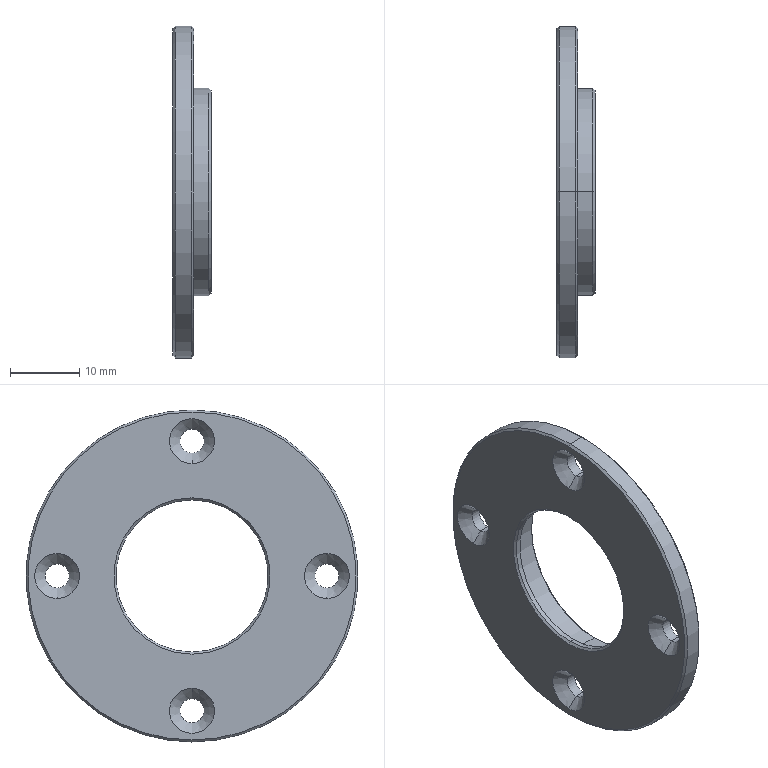Part | SolidWorks | features Chamfer 2, ICE 1, Revolution 1 | 1 solid | 38 faces | box 5.5 x 48 x 48 mm | volume 4296 mm3 | cone 18 | cylinder 16 | plane 4 | commonest cylinder face diameters 3.5 x8 22 x2 25.6 x2 30 x2 48 x2
STEP:
#1=CARTESIAN_POINT('',(0.3,0.,-11.));
#2=VERTEX_POINT('',#1);
#3=CARTESIAN_POINT('',(0.3,0.,11.));
#4=VERTEX_POINT('',#3);
#5=CARTESIAN_POINT('',(0.3,0.,0.));
#6=DIRECTION('',(-1.,0.,0.));
#7=DIRECTION('',(0.,0.,-1.));
#8=AXIS2_PLACEMENT_3D('',#5,#6,#7);
#9=CIRCLE('',#8,11.);
#10=EDGE_CURVE('',#2,#4,#9,.T.);
#11=ORIENTED_EDGE('',*,*,#10,.F.);
#12=CARTESIAN_POINT('',(0.,0.,-11.3));
#13=VERTEX_POINT('',#12);
#14=CARTESIAN_POINT('',(0.3,0.,-11.));
#15=DIRECTION('',(-0.7071,0.,-0.7071));
#16=VECTOR('',#15,1000.);
#17=LINE('',#14,#16);
#18=EDGE_CURVE('',#2,#13,#17,.T.);
#19=ORIENTED_EDGE('',*,*,#18,.T.);
#20=CARTESIAN_POINT('',(0.,0.,11.3));
#21=VERTEX_POINT('',#20);
#22=CARTESIAN_POINT('',(0.,0.,0.));
#23=DIRECTION('',(1.,0.,0.));
#24=DIRECTION('',(0.,0.,-1.));
#25=AXIS2_PLACEMENT_3D('',#22,#23,#24);
#26=CIRCLE('',#25,11.3);
#27=EDGE_CURVE('',#21,#13,#26,.T.);
#28=ORIENTED_EDGE('',*,*,#27,.F.);
#29=CARTESIAN_POINT('',(0.3,0.,11.));
#30=DIRECTION('',(-0.7071,0.,0.7071));
#31=VECTOR('',#30,1000.);
#32=LINE('',#29,#31);
#33=EDGE_CURVE('',#4,#21,#32,.T.);
#34=ORIENTED_EDGE('',*,*,#33,.F.);
#35=EDGE_LOOP('',(#11,#19,#28,#34));
#36=FACE_OUTER_BOUND('',#35,.T.);
#37=CARTESIAN_POINT('',(0.3,0.,0.));
#38=DIRECTION('',(-1.,0.,0.));
#39=DIRECTION('',(0.,0.,1.));
#40=AXIS2_PLACEMENT_3D('',#37,#38,#39);
#41=CONICAL_SURFACE('',#40,11.,0.7854);
#42=ADVANCED_FACE('',(#36),#41,.F.);
#43=CARTESIAN_POINT('',(0.,0.,23.7));
#44=VERTEX_POINT('',#43);
#45=CARTESIAN_POINT('',(0.,0.,-23.7));
#46=VERTEX_POINT('',#45);
#47=CARTESIAN_POINT('',(0.,0.,0.));
#48=DIRECTION('',(-1.,0.,0.));
#49=DIRECTION('',(0.,0.,-1.));
#50=AXIS2_PLACEMENT_3D('',#47,#48,#49);
#51=CIRCLE('',#50,23.7);
#52=EDGE_CURVE('',#44,#46,#51,.T.);
#53=ORIENTED_EDGE('',*,*,#52,.F.);
#54=CARTESIAN_POINT('',(0.3,0.,24.));
#55=VERTEX_POINT('',#54);
#56=CARTESIAN_POINT('',(0.,0.,23.7));
#57=DIRECTION('',(0.7071,0.,0.7071));
#58=VECTOR('',#57,1000.);
#59=LINE('',#56,#58);
#60=EDGE_CURVE('',#44,#55,#59,.T.);
#61=ORIENTED_EDGE('',*,*,#60,.T.);
#62=CARTESIAN_POINT('',(0.3,0.,-24.));
#63=VERTEX_POINT('',#62);
#64=CARTESIAN_POINT('',(0.3,0.,0.));
#65=DIRECTION('',(1.,0.,0.));
#66=DIRECTION('',(0.,0.,-1.));
#67=AXIS2_PLACEMENT_3D('',#64,#65,#66);
#68=CIRCLE('',#67,24.);
#69=EDGE_CURVE('',#63,#55,#68,.T.);
#70=ORIENTED_EDGE('',*,*,#69,.F.);
#71=CARTESIAN_POINT('',(0.,0.,-23.7));
#72=DIRECTION('',(0.7071,0.,-0.7071));
#73=VECTOR('',#72,1000.);
#74=LINE('',#71,#73);
#75=EDGE_CURVE('',#46,#63,#74,.T.);
#76=ORIENTED_EDGE('',*,*,#75,.F.);
#77=EDGE_LOOP('',(#53,#61,#70,#76));
#78=FACE_OUTER_BOUND('',#77,.T.);
#79=CARTESIAN_POINT('',(0.,0.,0.));
#80=DIRECTION('',(1.,0.,0.));
#81=DIRECTION('',(0.,0.,-1.));
#82=AXIS2_PLACEMENT_3D('',#79,#80,#81);
#83=CONICAL_SURFACE('',#82,23.7,0.7854);
#84=ADVANCED_FACE('',(#78),#83,.T.);
#85=CARTESIAN_POINT('',(3.,0.,-23.7));
#86=VERTEX_POINT('',#85);
#87=CARTESIAN_POINT('',(3.,0.,23.7));
#88=VERTEX_POINT('',#87);
#89=CARTESIAN_POINT('',(3.,0.,0.));
#90=DIRECTION('',(1.,0.,0.));
#91=DIRECTION('',(0.,0.,1.));
#92=AXIS2_PLACEMENT_3D('',#89,#90,#91);
#93=CIRCLE('',#92,23.7);
#94=EDGE_CURVE('',#86,#88,#93,.T.);
#95=ORIENTED_EDGE('',*,*,#94,.F.);
#96=CARTESIAN_POINT('',(2.7,0.,-24.));
#97=VERTEX_POINT('',#96);
#98=CARTESIAN_POINT('',(2.7,0.,-24.));
#99=DIRECTION('',(-0.7071,0.,-0.7071));
#100=VECTOR('',#99,1000.);
#101=LINE('',#98,#100);
#102=EDGE_CURVE('',#86,#97,#101,.T.);
#103=ORIENTED_EDGE('',*,*,#102,.T.);
#104=CARTESIAN_POINT('',(2.7,0.,24.));
#105=VERTEX_POINT('',#104);
#106=CARTESIAN_POINT('',(2.7,0.,0.));
#107=DIRECTION('',(-1.,0.,0.));
#108=DIRECTION('',(0.,0.,1.));
#109=AXIS2_PLACEMENT_3D('',#106,#107,#108);
#110=CIRCLE('',#109,24.);
#111=EDGE_CURVE('',#105,#97,#110,.T.);
#112=ORIENTED_EDGE('',*,*,#111,.F.);
#113=CARTESIAN_POINT('',(2.7,0.,24.));
#114=DIRECTION('',(-0.7071,0.,0.7071));
#115=VECTOR('',#114,1000.);
#116=LINE('',#113,#115);
#117=EDGE_CURVE('',#88,#105,#116,.T.);
#118=ORIENTED_EDGE('',*,*,#117,.F.);
#119=EDGE_LOOP('',(#95,#103,#112,#118));
#120=FACE_OUTER_BOUND('',#119,.T.);
#121=CARTESIAN_POINT('',(2.7,0.,0.));
#122=DIRECTION('',(-1.,0.,0.));
#123=DIRECTION('',(0.,0.,1.));
#124=AXIS2_PLACEMENT_3D('',#121,#122,#123);
#125=CONICAL_SURFACE('',#124,24.,0.7854);
#126=ADVANCED_FACE('',(#120),#125,.T.);
#127=CARTESIAN_POINT('',(5.2,0.,12.8));
#128=VERTEX_POINT('',#127);
#129=CARTESIAN_POINT('',(5.2,0.,-12.8));
#130=VERTEX_POINT('',#129);
#131=CARTESIAN_POINT('',(5.2,0.,0.));
#132=DIRECTION('',(1.,0.,0.));
#133=DIRECTION('',(0.,0.,1.));
#134=AXIS2_PLACEMENT_3D('',#131,#132,#133);
#135=CIRCLE('',#134,12.8);
#136=EDGE_CURVE('',#128,#130,#135,.T.);
#137=ORIENTED_EDGE('',*,*,#136,.F.);
#138=CARTESIAN_POINT('',(5.5,0.,13.1));
#139=VERTEX_POINT('',#138);
#140=CARTESIAN_POINT('',(5.5,0.,13.1));
#141=DIRECTION('',(0.7071,0.,0.7071));
#142=VECTOR('',#141,1000.);
#143=LINE('',#140,#142);
#144=EDGE_CURVE('',#128,#139,#143,.T.);
#145=ORIENTED_EDGE('',*,*,#144,.T.);
#146=CARTESIAN_POINT('',(5.5,0.,-13.1));
#147=VERTEX_POINT('',#146);
#148=CARTESIAN_POINT('',(5.5,0.,0.));
#149=DIRECTION('',(-1.,0.,0.));
#150=DIRECTION('',(0.,0.,1.));
#151=AXIS2_PLACEMENT_3D('',#148,#149,#150);
#152=CIRCLE('',#151,13.1);
#153=EDGE_CURVE('',#147,#139,#152,.T.);
#154=ORIENTED_EDGE('',*,*,#153,.F.);
#155=CARTESIAN_POINT('',(5.5,0.,-13.1));
#156=DIRECTION('',(0.7071,0.,-0.7071));
#157=VECTOR('',#156,1000.);
#158=LINE('',#155,#157);
#159=EDGE_CURVE('',#130,#147,#158,.T.);
#160=ORIENTED_EDGE('',*,*,#159,.F.);
#161=EDGE_LOOP('',(#137,#145,#154,#160));
#162=FACE_OUTER_BOUND('',#161,.T.);
#163=CARTESIAN_POINT('',(5.5,0.,0.));
#164=DIRECTION('',(1.,0.,0.));
#165=DIRECTION('',(0.,0.,-1.));
#166=AXIS2_PLACEMENT_3D('',#163,#164,#165);
#167=CONICAL_SURFACE('',#166,13.1,0.7854);
#168=ADVANCED_FACE('',(#162),#167,.F.);
#169=CARTESIAN_POINT('',(5.5,0.,-14.7));
#170=VERTEX_POINT('',#169);
#171=CARTESIAN_POINT('',(5.5,0.,14.7));
#172=VERTEX_POINT('',#171);
#173=CARTESIAN_POINT('',(5.5,0.,0.));
#174=DIRECTION('',(1.,0.,0.));
#175=DIRECTION('',(0.,0.,1.));
#176=AXIS2_PLACEMENT_3D('',#173,#174,#175);
#177=CIRCLE('',#176,14.7);
#178=EDGE_CURVE('',#170,#172,#177,.T.);
#179=ORIENTED_EDGE('',*,*,#178,.F.);
#180=CARTESIAN_POINT('',(5.2,0.,-15.));
#181=VERTEX_POINT('',#180);
#182=CARTESIAN_POINT('',(5.2,0.,-15.));
#183=DIRECTION('',(-0.7071,0.,-0.7071));
#184=VECTOR('',#183,1000.);
#185=LINE('',#182,#184);
#186=EDGE_CURVE('',#170,#181,#185,.T.);
#187=ORIENTED_EDGE('',*,*,#186,.T.);
#188=CARTESIAN_POINT('',(5.2,0.,15.));
#189=VERTEX_POINT('',#188);
#190=CARTESIAN_POINT('',(5.2,0.,0.));
#191=DIRECTION('',(-1.,0.,0.));
#192=DIRECTION('',(0.,0.,1.));
#193=AXIS2_PLACEMENT_3D('',#190,#191,#192);
#194=CIRCLE('',#193,15.);
#195=EDGE_CURVE('',#189,#181,#194,.T.);
#196=ORIENTED_EDGE('',*,*,#195,.F.);
#197=CARTESIAN_POINT('',(5.2,0.,15.));
#198=DIRECTION('',(-0.7071,0.,0.7071));
#199=VECTOR('',#198,1000.);
#200=LINE('',#197,#199);
#201=EDGE_CURVE('',#172,#189,#200,.T.);
#202=ORIENTED_EDGE('',*,*,#201,.F.);
#203=EDGE_LOOP('',(#179,#187,#196,#202));
#204=FACE_OUTER_BOUND('',#203,.T.);
#205=CARTESIAN_POINT('',(5.2,0.,0.));
#206=DIRECTION('',(-1.,0.,0.));
#207=DIRECTION('',(0.,0.,1.));
#208=AXIS2_PLACEMENT_3D('',#205,#206,#207);
#209=CONICAL_SURFACE('',#208,15.,0.7854);
#210=ADVANCED_FACE('',(#204),#209,.T.);
#211=CARTESIAN_POINT('',(1.5,0.,-21.25));
#212=VERTEX_POINT('',#211);
#213=CARTESIAN_POINT('',(1.5,0.,-17.75));
#214=VERTEX_POINT('',#213);
#215=CARTESIAN_POINT('',(1.5,0.,-19.5));
#216=DIRECTION('',(-1.,0.,0.));
#217=DIRECTION('',(0.,0.,-1.));
#218=AXIS2_PLACEMENT_3D('',#215,#216,#217);
#219=CIRCLE('',#218,1.75);
#220=EDGE_CURVE('',#212,#214,#219,.T.);
#221=ORIENTED_EDGE('',*,*,#220,.F.);
#222=CARTESIAN_POINT('',(0.,0.,-22.75));
#223=VERTEX_POINT('',#222);
#224=CARTESIAN_POINT('',(1.5,0.,-21.25));
#225=DIRECTION('',(-0.7071,0.,-0.7071));
#226=VECTOR('',#225,1000.);
#227=LINE('',#224,#226);
#228=EDGE_CURVE('',#212,#223,#227,.T.);
#229=ORIENTED_EDGE('',*,*,#228,.T.);
#230=CARTESIAN_POINT('',(0.,0.,-16.25));
#231=VERTEX_POINT('',#230);
#232=CARTESIAN_POINT('',(0.,0.,-19.5));
#233=DIRECTION('',(1.,0.,0.));
#234=DIRECTION('',(0.,0.,-1.));
#235=AXIS2_PLACEMENT_3D('',#232,#233,#234);
#236=CIRCLE('',#235,3.25);
#237=EDGE_CURVE('',#231,#223,#236,.T.);
#238=ORIENTED_EDGE('',*,*,#237,.F.);
#239=CARTESIAN_POINT('',(1.5,0.,-17.75));
#240=DIRECTION('',(-0.7071,0.,0.7071));
#241=VECTOR('',#240,1000.);
#242=LINE('',#239,#241);
#243=EDGE_CURVE('',#214,#231,#242,.T.);
#244=ORIENTED_EDGE('',*,*,#243,.F.);
#245=EDGE_LOOP('',(#221,#229,#238,#244));
#246=FACE_OUTER_BOUND('',#245,.T.);
#247=CARTESIAN_POINT('',(1.5,0.,-19.5));
#248=DIRECTION('',(-1.,0.,0.));
#249=DIRECTION('',(0.,0.,1.));
#250=AXIS2_PLACEMENT_3D('',#247,#248,#249);
#251=CONICAL_SURFACE('',#250,1.75,0.7854);
#252=ADVANCED_FACE('',(#246),#251,.F.);
#253=CARTESIAN_POINT('',(1.5,19.5,-1.75));
#254=VERTEX_POINT('',#253);
#255=CARTESIAN_POINT('',(1.5,19.5,1.75));
#256=VERTEX_POINT('',#255);
#257=CARTESIAN_POINT('',(1.5,19.5,0.));
#258=DIRECTION('',(-1.,0.,0.));
#259=DIRECTION('',(0.,0.,-1.));
#260=AXIS2_PLACEMENT_3D('',#257,#258,#259);
#261=CIRCLE('',#260,1.75);
#262=EDGE_CURVE('',#254,#256,#261,.T.);
#263=ORIENTED_EDGE('',*,*,#262,.F.);
#264=CARTESIAN_POINT('',(0.,19.5,-3.25));
#265=VERTEX_POINT('',#264);
#266=CARTESIAN_POINT('',(1.5,19.5,-1.75));
#267=DIRECTION('',(-0.7071,0.,-0.7071));
#268=VECTOR('',#267,1000.);
#269=LINE('',#266,#268);
#270=EDGE_CURVE('',#254,#265,#269,.T.);
#271=ORIENTED_EDGE('',*,*,#270,.T.);
#272=CARTESIAN_POINT('',(0.,19.5,3.25));
#273=VERTEX_POINT('',#272);
#274=CARTESIAN_POINT('',(0.,19.5,0.));
#275=DIRECTION('',(1.,0.,0.));
#276=DIRECTION('',(0.,0.,-1.));
#277=AXIS2_PLACEMENT_3D('',#274,#275,#276);
#278=CIRCLE('',#277,3.25);
#279=EDGE_CURVE('',#273,#265,#278,.T.);
#280=ORIENTED_EDGE('',*,*,#279,.F.);
#281=CARTESIAN_POINT('',(1.5,19.5,1.75));
#282=DIRECTION('',(-0.7071,0.,0.7071));
#283=VECTOR('',#282,1000.);
#284=LINE('',#281,#283);
#285=EDGE_CURVE('',#256,#273,#284,.T.);
#286=ORIENTED_EDGE('',*,*,#285,.F.);
#287=EDGE_LOOP('',(#263,#271,#280,#286));
#288=FACE_OUTER_BOUND('',#287,.T.);
#289=CARTESIAN_POINT('',(1.5,19.5,0.));
#290=DIRECTION('',(-1.,0.,0.));
#291=DIRECTION('',(0.,0.,1.));
#292=AXIS2_PLACEMENT_3D('',#289,#290,#291);
#293=CONICAL_SURFACE('',#292,1.75,0.7854);
#294=ADVANCED_FACE('',(#288),#293,.F.);
#295=CARTESIAN_POINT('',(1.5,-19.5,-1.75));
#296=VERTEX_POINT('',#295);
#297=CARTESIAN_POINT('',(1.5,-19.5,1.75));
#298=VERTEX_POINT('',#297);
#299=CARTESIAN_POINT('',(1.5,-19.5,0.));
#300=DIRECTION('',(-1.,0.,0.));
#301=DIRECTION('',(0.,0.,-1.));
#302=AXIS2_PLACEMENT_3D('',#299,#300,#301);
#303=CIRCLE('',#302,1.75);
#304=EDGE_CURVE('',#296,#298,#303,.T.);
#305=ORIENTED_EDGE('',*,*,#304,.F.);
#306=CARTESIAN_POINT('',(0.,-19.5,-3.25));
#307=VERTEX_POINT('',#306);
#308=CARTESIAN_POINT('',(1.5,-19.5,-1.75));
#309=DIRECTION('',(-0.7071,0.,-0.7071));
#310=VECTOR('',#309,1000.);
#311=LINE('',#308,#310);
#312=EDGE_CURVE('',#296,#307,#311,.T.);
#313=ORIENTED_EDGE('',*,*,#312,.T.);
#314=CARTESIAN_POINT('',(0.,-19.5,3.25));
#315=VERTEX_POINT('',#314);
#316=CARTESIAN_POINT('',(0.,-19.5,0.));
#317=DIRECTION('',(1.,0.,0.));
#318=DIRECTION('',(0.,0.,-1.));
#319=AXIS2_PLACEMENT_3D('',#316,#317,#318);
#320=CIRCLE('',#319,3.25);
#321=EDGE_CURVE('',#315,#307,#320,.T.);
#322=ORIENTED_EDGE('',*,*,#321,.F.);
#323=CARTESIAN_POINT('',(1.5,-19.5,1.75));
#324=DIRECTION('',(-0.7071,0.,0.7071));
#325=VECTOR('',#324,1000.);
#326=LINE('',#323,#325);
#327=EDGE_CURVE('',#298,#315,#326,.T.);
#328=ORIENTED_EDGE('',*,*,#327,.F.);
#329=EDGE_LOOP('',(#305,#313,#322,#328));
#330=FACE_OUTER_BOUND('',#329,.T.);
#331=CARTESIAN_POINT('',(1.5,-19.5,0.));
#332=DIRECTION('',(-1.,0.,0.));
#333=DIRECTION('',(0.,0.,1.));
#334=AXIS2_PLACEMENT_3D('',#331,#332,#333);
#335=CONICAL_SURFACE('',#334,1.75,0.7854);
#336=ADVANCED_FACE('',(#330),#335,.F.);
#337=CARTESIAN_POINT('',(1.5,0.,17.75));
#338=VERTEX_POINT('',#337);
#339=CARTESIAN_POINT('',(1.5,0.,21.25));
#340=VERTEX_POINT('',#339);
#341=CARTESIAN_POINT('',(1.5,0.,19.5));
#342=DIRECTION('',(-1.,0.,0.));
#343=DIRECTION('',(0.,0.,-1.));
#344=AXIS2_PLACEMENT_3D('',#341,#342,#343);
#345=CIRCLE('',#344,1.75);
#346=EDGE_CURVE('',#338,#340,#345,.T.);
#347=ORIENTED_EDGE('',*,*,#346,.F.);
#348=CARTESIAN_POINT('',(0.,0.,16.25));
#349=VERTEX_POINT('',#348);
#350=CARTESIAN_POINT('',(1.5,0.,17.75));
#351=DIRECTION('',(-0.7071,0.,-0.7071));
#352=VECTOR('',#351,1000.);
#353=LINE('',#350,#352);
#354=EDGE_CURVE('',#338,#349,#353,.T.);
#355=ORIENTED_EDGE('',*,*,#354,.T.);
#356=CARTESIAN_POINT('',(0.,0.,22.75));
#357=VERTEX_POINT('',#356);
#358=CARTESIAN_POINT('',(0.,0.,19.5));
#359=DIRECTION('',(1.,0.,0.));
#360=DIRECTION('',(0.,0.,-1.));
#361=AXIS2_PLACEMENT_3D('',#358,#359,#360);
#362=CIRCLE('',#361,3.25);
#363=EDGE_CURVE('',#357,#349,#362,.T.);
#364=ORIENTED_EDGE('',*,*,#363,.F.);
#365=CARTESIAN_POINT('',(1.5,0.,21.25));
#366=DIRECTION('',(-0.7071,0.,0.7071));
#367=VECTOR('',#366,1000.);
#368=LINE('',#365,#367);
#369=EDGE_CURVE('',#340,#357,#368,.T.);
#370=ORIENTED_EDGE('',*,*,#369,.F.);
#371=EDGE_LOOP('',(#347,#355,#364,#370));
#372=FACE_OUTER_BOUND('',#371,.T.);
#373=CARTESIAN_POINT('',(1.5,0.,19.5));
#374=DIRECTION('',(-1.,0.,0.));
#375=DIRECTION('',(0.,0.,1.));
#376=AXIS2_PLACEMENT_3D('',#373,#374,#375);
#377=CONICAL_SURFACE('',#376,1.75,0.7854);
#378=ADVANCED_FACE('',(#372),#377,.F.);
#379=ORIENTED_EDGE('',*,*,#262,.T.);
#380=CARTESIAN_POINT('',(3.,19.5,1.75));
#381=VERTEX_POINT('',#380);
#382=CARTESIAN_POINT('',(-4.95,19.5,1.75));
#383=DIRECTION('',(1.,0.,0.));
#384=VECTOR('',#383,1000.);
#385=LINE('',#382,#384);
#386=EDGE_CURVE('',#256,#381,#385,.T.);
#387=ORIENTED_EDGE('',*,*,#386,.T.);
#388=CARTESIAN_POINT('',(3.,19.5,-1.75));
#389=VERTEX_POINT('',#388);
#390=CARTESIAN_POINT('',(3.,19.5,0.));
#391=DIRECTION('',(1.,0.,0.));
#392=DIRECTION('',(0.,0.,-1.));
#393=AXIS2_PLACEMENT_3D('',#390,#391,#392);
#394=CIRCLE('',#393,1.75);
#395=EDGE_CURVE('',#381,#389,#394,.T.);
#396=ORIENTED_EDGE('',*,*,#395,.T.);
#397=CARTESIAN_POINT('',(-4.95,19.5,-1.75));
#398=DIRECTION('',(1.,0.,0.));
#399=VECTOR('',#398,1000.);
#400=LINE('',#397,#399);
#401=EDGE_CURVE('',#254,#389,#400,.T.);
#402=ORIENTED_EDGE('',*,*,#401,.F.);
#403=EDGE_LOOP('',(#379,#387,#396,#402));
#404=FACE_OUTER_BOUND('',#403,.T.);
#405=CARTESIAN_POINT('',(-4.95,19.5,0.));
#406=DIRECTION('',(1.,0.,0.));
#407=DIRECTION('',(0.,0.,-1.));
#408=AXIS2_PLACEMENT_3D('',#405,#406,#407);
#409=CYLINDRICAL_SURFACE('',#408,1.75);
#410=ADVANCED_FACE('',(#404),#409,.F.);
#411=ORIENTED_EDGE('',*,*,#220,.T.);
#412=CARTESIAN_POINT('',(3.,0.,-17.75));
#413=VERTEX_POINT('',#412);
#414=CARTESIAN_POINT('',(-4.95,0.,-17.75));
#415=DIRECTION('',(1.,0.,0.));
#416=VECTOR('',#415,1000.);
#417=LINE('',#414,#416);
#418=EDGE_CURVE('',#214,#413,#417,.T.);
#419=ORIENTED_EDGE('',*,*,#418,.T.);
#420=CARTESIAN_POINT('',(3.,0.,-21.25));
#421=VERTEX_POINT('',#420);
#422=CARTESIAN_POINT('',(3.,0.,-19.5));
#423=DIRECTION('',(1.,0.,0.));
#424=DIRECTION('',(0.,0.,-1.));
#425=AXIS2_PLACEMENT_3D('',#422,#423,#424);
#426=CIRCLE('',#425,1.75);
#427=EDGE_CURVE('',#413,#421,#426,.T.);
#428=ORIENTED_EDGE('',*,*,#427,.T.);
#429=CARTESIAN_POINT('',(-4.95,0.,-21.25));
#430=DIRECTION('',(1.,0.,0.));
#431=VECTOR('',#430,1000.);
#432=LINE('',#429,#431);
#433=EDGE_CURVE('',#212,#421,#432,.T.);
#434=ORIENTED_EDGE('',*,*,#433,.F.);
#435=EDGE_LOOP('',(#411,#419,#428,#434));
#436=FACE_OUTER_BOUND('',#435,.T.);
#437=CARTESIAN_POINT('',(-4.95,0.,-19.5));
#438=DIRECTION('',(1.,0.,0.));
#439=DIRECTION('',(0.,0.,-1.));
#440=AXIS2_PLACEMENT_3D('',#437,#438,#439);
#441=CYLINDRICAL_SURFACE('',#440,1.75);
#442=ADVANCED_FACE('',(#436),#441,.F.);
#443=ORIENTED_EDGE('',*,*,#304,.T.);
#444=CARTESIAN_POINT('',(3.,-19.5,1.75));
#445=VERTEX_POINT('',#444);
#446=CARTESIAN_POINT('',(-4.95,-19.5,1.75));
#447=DIRECTION('',(1.,0.,0.));
#448=VECTOR('',#447,1000.);
#449=LINE('',#446,#448);
#450=EDGE_CURVE('',#298,#445,#449,.T.);
#451=ORIENTED_EDGE('',*,*,#450,.T.);
#452=CARTESIAN_POINT('',(3.,-19.5,-1.75));
#453=VERTEX_POINT('',#452);
#454=CARTESIAN_POINT('',(3.,-19.5,0.));
#455=DIRECTION('',(1.,0.,0.));
#456=DIRECTION('',(0.,0.,-1.));
#457=AXIS2_PLACEMENT_3D('',#454,#455,#456);
#458=CIRCLE('',#457,1.75);
#459=EDGE_CURVE('',#445,#453,#458,.T.);
#460=ORIENTED_EDGE('',*,*,#459,.T.);
#461=CARTESIAN_POINT('',(-4.95,-19.5,-1.75));
#462=DIRECTION('',(1.,0.,0.));
#463=VECTOR('',#462,1000.);
#464=LINE('',#461,#463);
#465=EDGE_CURVE('',#296,#453,#464,.T.);
#466=ORIENTED_EDGE('',*,*,#465,.F.);
#467=EDGE_LOOP('',(#443,#451,#460,#466));
#468=FACE_OUTER_BOUND('',#467,.T.);
#469=CARTESIAN_POINT('',(-4.95,-19.5,0.));
#470=DIRECTION('',(1.,0.,0.));
#471=DIRECTION('',(0.,0.,-1.));
#472=AXIS2_PLACEMENT_3D('',#469,#470,#471);
#473=CYLINDRICAL_SURFACE('',#472,1.75);
#474=ADVANCED_FACE('',(#468),#473,.F.);
#475=ORIENTED_EDGE('',*,*,#346,.T.);
#476=CARTESIAN_POINT('',(3.,0.,21.25));
#477=VERTEX_POINT('',#476);
#478=CARTESIAN_POINT('',(-4.95,0.,21.25));
#479=DIRECTION('',(1.,0.,0.));
#480=VECTOR('',#479,1000.);
#481=LINE('',#478,#480);
#482=EDGE_CURVE('',#340,#477,#481,.T.);
#483=ORIENTED_EDGE('',*,*,#482,.T.);
#484=CARTESIAN_POINT('',(3.,0.,17.75));
#485=VERTEX_POINT('',#484);
#486=CARTESIAN_POINT('',(3.,0.,19.5));
#487=DIRECTION('',(1.,0.,0.));
#488=DIRECTION('',(0.,0.,-1.));
#489=AXIS2_PLACEMENT_3D('',#486,#487,#488);
#490=CIRCLE('',#489,1.75);
#491=EDGE_CURVE('',#477,#485,#490,.T.);
#492=ORIENTED_EDGE('',*,*,#491,.T.);
#493=CARTESIAN_POINT('',(-4.95,0.,17.75));
#494=DIRECTION('',(1.,0.,0.));
#495=VECTOR('',#494,1000.);
#496=LINE('',#493,#495);
#497=EDGE_CURVE('',#338,#485,#496,.T.);
#498=ORIENTED_EDGE('',*,*,#497,.F.);
#499=EDGE_LOOP('',(#475,#483,#492,#498));
#500=FACE_OUTER_BOUND('',#499,.T.);
#501=CARTESIAN_POINT('',(-4.95,0.,19.5));
#502=DIRECTION('',(1.,0.,0.));
#503=DIRECTION('',(0.,0.,-1.));
#504=AXIS2_PLACEMENT_3D('',#501,#502,#503);
#505=CYLINDRICAL_SURFACE('',#504,1.75);
#506=ADVANCED_FACE('',(#500),#505,.F.);
#507=ORIENTED_EDGE('',*,*,#111,.T.);
#508=CARTESIAN_POINT('',(0.,0.,-24.));
#509=DIRECTION('',(-1.,0.,0.));
#510=VECTOR('',#509,1000.);
#511=LINE('',#508,#510);
#512=EDGE_CURVE('',#97,#63,#511,.T.);
#513=ORIENTED_EDGE('',*,*,#512,.T.);
#514=ORIENTED_EDGE('',*,*,#69,.T.);
#515=CARTESIAN_POINT('',(0.,0.,24.));
#516=DIRECTION('',(-1.,0.,0.));
#517=VECTOR('',#516,1000.);
#518=LINE('',#515,#517);
#519=EDGE_CURVE('',#105,#55,#518,.T.);
#520=ORIENTED_EDGE('',*,*,#519,.F.);
#521=EDGE_LOOP('',(#507,#513,#514,#520));
#522=FACE_OUTER_BOUND('',#521,.T.);
#523=CARTESIAN_POINT('',(0.,0.,0.));
#524=DIRECTION('',(-1.,0.,0.));
#525=DIRECTION('',(0.,0.,1.));
#526=AXIS2_PLACEMENT_3D('',#523,#524,#525);
#527=CYLINDRICAL_SURFACE('',#526,24.);
#528=ADVANCED_FACE('',(#522),#527,.T.);
#529=CARTESIAN_POINT('',(1.,0.,-11.));
#530=VERTEX_POINT('',#529);
#531=CARTESIAN_POINT('',(1.,0.,11.));
#532=VERTEX_POINT('',#531);
#533=CARTESIAN_POINT('',(1.,0.,0.));
#534=DIRECTION('',(-1.,0.,0.));
#535=DIRECTION('',(0.,0.,1.));
#536=AXIS2_PLACEMENT_3D('',#533,#534,#535);
#537=CIRCLE('',#536,11.);
#538=EDGE_CURVE('',#530,#532,#537,.T.);
#539=ORIENTED_EDGE('',*,*,#538,.F.);
#540=CARTESIAN_POINT('',(0.,0.,-11.));
#541=DIRECTION('',(-1.,0.,0.));
#542=VECTOR('',#541,1000.);
#543=LINE('',#540,#542);
#544=EDGE_CURVE('',#530,#2,#543,.T.);
#545=ORIENTED_EDGE('',*,*,#544,.T.);
#546=ORIENTED_EDGE('',*,*,#10,.T.);
#547=CARTESIAN_POINT('',(0.,0.,11.));
#548=DIRECTION('',(-1.,0.,0.));
#549=VECTOR('',#548,1000.);
#550=LINE('',#547,#549);
#551=EDGE_CURVE('',#532,#4,#550,.T.);
#552=ORIENTED_EDGE('',*,*,#551,.F.);
#553=EDGE_LOOP('',(#539,#545,#546,#552));
#554=FACE_OUTER_BOUND('',#553,.T.);
#555=CARTESIAN_POINT('',(0.,0.,0.));
#556=DIRECTION('',(-1.,0.,0.));
#557=DIRECTION('',(0.,0.,1.));
#558=AXIS2_PLACEMENT_3D('',#555,#556,#557);
#559=CYLINDRICAL_SURFACE('',#558,11.);
#560=ADVANCED_FACE('',(#554),#559,.F.);
#561=ORIENTED_EDGE('',*,*,#136,.T.);
#562=CARTESIAN_POINT('',(1.,0.,-12.8));
#563=VERTEX_POINT('',#562);
#564=CARTESIAN_POINT('',(0.,0.,-12.8));
#565=DIRECTION('',(-1.,0.,0.));
#566=VECTOR('',#565,1000.);
#567=LINE('',#564,#566);
#568=EDGE_CURVE('',#130,#563,#567,.T.);
#569=ORIENTED_EDGE('',*,*,#568,.T.);
#570=CARTESIAN_POINT('',(1.,0.,12.8));
#571=VERTEX_POINT('',#570);
#572=CARTESIAN_POINT('',(1.,0.,0.));
#573=DIRECTION('',(-1.,0.,0.));
#574=DIRECTION('',(0.,0.,1.));
#575=AXIS2_PLACEMENT_3D('',#572,#573,#574);
#576=CIRCLE('',#575,12.8);
#577=EDGE_CURVE('',#563,#571,#576,.T.);
#578=ORIENTED_EDGE('',*,*,#577,.T.);
#579=CARTESIAN_POINT('',(0.,0.,12.8));
#580=DIRECTION('',(-1.,0.,0.));
#581=VECTOR('',#580,1000.);
#582=LINE('',#579,#581);
#583=EDGE_CURVE('',#128,#571,#582,.T.);
#584=ORIENTED_EDGE('',*,*,#583,.F.);
#585=EDGE_LOOP('',(#561,#569,#578,#584));
#586=FACE_OUTER_BOUND('',#585,.T.);
#587=CARTESIAN_POINT('',(0.,0.,0.));
#588=DIRECTION('',(-1.,0.,0.));
#589=DIRECTION('',(0.,0.,1.));
#590=AXIS2_PLACEMENT_3D('',#587,#588,#589);
#591=CYLINDRICAL_SURFACE('',#590,12.8);
#592=ADVANCED_FACE('',(#586),#591,.F.);
#593=ORIENTED_EDGE('',*,*,#195,.T.);
#594=CARTESIAN_POINT('',(3.,0.,-15.));
#595=VERTEX_POINT('',#594);
#596=CARTESIAN_POINT('',(0.,0.,-15.));
#597=DIRECTION('',(-1.,0.,0.));
#598=VECTOR('',#597,1000.);
#599=LINE('',#596,#598);
#600=EDGE_CURVE('',#181,#595,#599,.T.);
#601=ORIENTED_EDGE('',*,*,#600,.T.);
#602=CARTESIAN_POINT('',(3.,0.,15.));
#603=VERTEX_POINT('',#602);
#604=CARTESIAN_POINT('',(3.,0.,0.));
#605=DIRECTION('',(-1.,0.,0.));
#606=DIRECTION('',(0.,0.,1.));
#607=AXIS2_PLACEMENT_3D('',#604,#605,#606);
#608=CIRCLE('',#607,15.);
#609=EDGE_CURVE('',#603,#595,#608,.T.);
#610=ORIENTED_EDGE('',*,*,#609,.F.);
#611=CARTESIAN_POINT('',(0.,0.,15.));
#612=DIRECTION('',(-1.,0.,0.));
#613=VECTOR('',#612,1000.);
#614=LINE('',#611,#613);
#615=EDGE_CURVE('',#189,#603,#614,.T.);
#616=ORIENTED_EDGE('',*,*,#615,.F.);
#617=EDGE_LOOP('',(#593,#601,#610,#616));
#618=FACE_OUTER_BOUND('',#617,.T.);
#619=CARTESIAN_POINT('',(0.,0.,0.));
#620=DIRECTION('',(-1.,0.,0.));
#621=DIRECTION('',(0.,0.,1.));
#622=AXIS2_PLACEMENT_3D('',#619,#620,#621);
#623=CYLINDRICAL_SURFACE('',#622,15.);
#624=ADVANCED_FACE('',(#618),#623,.T.);
#625=ORIENTED_EDGE('',*,*,#600,.F.);
#626=CARTESIAN_POINT('',(5.2,0.,0.));
#627=DIRECTION('',(-1.,0.,0.));
#628=DIRECTION('',(0.,0.,1.));
#629=AXIS2_PLACEMENT_3D('',#626,#627,#628);
#630=CIRCLE('',#629,15.);
#631=EDGE_CURVE('',#181,#189,#630,.T.);
#632=ORIENTED_EDGE('',*,*,#631,.T.);
#633=ORIENTED_EDGE('',*,*,#615,.T.);
#634=CARTESIAN_POINT('',(3.,0.,0.));
#635=DIRECTION('',(-1.,0.,0.));
#636=DIRECTION('',(0.,0.,1.));
#637=AXIS2_PLACEMENT_3D('',#634,#635,#636);
#638=CIRCLE('',#637,15.);
#639=EDGE_CURVE('',#595,#603,#638,.T.);
#640=ORIENTED_EDGE('',*,*,#639,.F.);
#641=EDGE_LOOP('',(#625,#632,#633,#640));
#642=FACE_OUTER_BOUND('',#641,.T.);
#643=CARTESIAN_POINT('',(0.,0.,0.));
#644=DIRECTION('',(-1.,0.,0.));
#645=DIRECTION('',(0.,0.,1.));
#646=AXIS2_PLACEMENT_3D('',#643,#644,#645);
#647=CYLINDRICAL_SURFACE('',#646,15.);
#648=ADVANCED_FACE('',(#642),#647,.T.);
#649=CARTESIAN_POINT('',(5.5,0.,0.));
#650=DIRECTION('',(1.,0.,0.));
#651=DIRECTION('',(0.,0.,1.));
#652=AXIS2_PLACEMENT_3D('',#649,#650,#651);
#653=CIRCLE('',#652,14.7);
#654=EDGE_CURVE('',#172,#170,#653,.T.);
#655=ORIENTED_EDGE('',*,*,#654,.T.);
#656=ORIENTED_EDGE('',*,*,#178,.T.);
#657=EDGE_LOOP('',(#655,#656));
#658=FACE_OUTER_BOUND('',#657,.T.);
#659=ORIENTED_EDGE('',*,*,#153,.T.);
#660=CARTESIAN_POINT('',(5.5,0.,0.));
#661=DIRECTION('',(-1.,0.,0.));
#662=DIRECTION('',(0.,0.,1.));
#663=AXIS2_PLACEMENT_3D('',#660,#661,#662);
#664=CIRCLE('',#663,13.1);
#665=EDGE_CURVE('',#139,#147,#664,.T.);
#666=ORIENTED_EDGE('',*,*,#665,.T.);
#667=EDGE_LOOP('',(#659,#666));
#668=FACE_BOUND('',#667,.T.);
#669=CARTESIAN_POINT('',(5.5,15.,0.));
#670=DIRECTION('',(-1.,0.,0.));
#671=DIRECTION('',(0.,0.,1.));
#672=AXIS2_PLACEMENT_3D('',#669,#670,#671);
#673=PLANE('',#672);
#674=ADVANCED_FACE('',(#658,#668),#673,.F.);
#675=ORIENTED_EDGE('',*,*,#568,.F.);
#676=CARTESIAN_POINT('',(5.2,0.,0.));
#677=DIRECTION('',(1.,0.,0.));
#678=DIRECTION('',(0.,0.,1.));
#679=AXIS2_PLACEMENT_3D('',#676,#677,#678);
#680=CIRCLE('',#679,12.8);
#681=EDGE_CURVE('',#130,#128,#680,.T.);
#682=ORIENTED_EDGE('',*,*,#681,.T.);
#683=ORIENTED_EDGE('',*,*,#583,.T.);
#684=CARTESIAN_POINT('',(1.,0.,0.));
#685=DIRECTION('',(-1.,0.,0.));
#686=DIRECTION('',(0.,0.,1.));
#687=AXIS2_PLACEMENT_3D('',#684,#685,#686);
#688=CIRCLE('',#687,12.8);
#689=EDGE_CURVE('',#571,#563,#688,.T.);
#690=ORIENTED_EDGE('',*,*,#689,.T.);
#691=EDGE_LOOP('',(#675,#682,#683,#690));
#692=FACE_OUTER_BOUND('',#691,.T.);
#693=CARTESIAN_POINT('',(0.,0.,0.));
#694=DIRECTION('',(-1.,0.,0.));
#695=DIRECTION('',(0.,0.,1.));
#696=AXIS2_PLACEMENT_3D('',#693,#694,#695);
#697=CYLINDRICAL_SURFACE('',#696,12.8);
#698=ADVANCED_FACE('',(#692),#697,.F.);
#699=ORIENTED_EDGE('',*,*,#689,.F.);
#700=ORIENTED_EDGE('',*,*,#577,.F.);
#701=EDGE_LOOP('',(#699,#700));
#702=FACE_OUTER_BOUND('',#701,.T.);
#703=CARTESIAN_POINT('',(1.,0.,0.));
#704=DIRECTION('',(-1.,0.,0.));
#705=DIRECTION('',(0.,0.,1.));
#706=AXIS2_PLACEMENT_3D('',#703,#704,#705);
#707=CIRCLE('',#706,11.);
#708=EDGE_CURVE('',#532,#530,#707,.T.);
#709=ORIENTED_EDGE('',*,*,#708,.T.);
#710=ORIENTED_EDGE('',*,*,#538,.T.);
#711=EDGE_LOOP('',(#709,#710));
#712=FACE_BOUND('',#711,.T.);
#713=CARTESIAN_POINT('',(1.,12.8,0.));
#714=DIRECTION('',(-1.,0.,0.));
#715=DIRECTION('',(0.,0.,1.));
#716=AXIS2_PLACEMENT_3D('',#713,#714,#715);
#717=PLANE('',#716);
#718=ADVANCED_FACE('',(#702,#712),#717,.F.);
#719=ORIENTED_EDGE('',*,*,#544,.F.);
#720=ORIENTED_EDGE('',*,*,#708,.F.);
#721=ORIENTED_EDGE('',*,*,#551,.T.);
#722=CARTESIAN_POINT('',(0.3,0.,0.));
#723=DIRECTION('',(-1.,0.,0.));
#724=DIRECTION('',(0.,0.,-1.));
#725=AXIS2_PLACEMENT_3D('',#722,#723,#724);
#726=CIRCLE('',#725,11.);
#727=EDGE_CURVE('',#4,#2,#726,.T.);
#728=ORIENTED_EDGE('',*,*,#727,.T.);
#729=EDGE_LOOP('',(#719,#720,#721,#728));
#730=FACE_OUTER_BOUND('',#729,.T.);
#731=CARTESIAN_POINT('',(0.,0.,0.));
#732=DIRECTION('',(-1.,0.,0.));
#733=DIRECTION('',(0.,0.,1.));
#734=AXIS2_PLACEMENT_3D('',#731,#732,#733);
#735=CYLINDRICAL_SURFACE('',#734,11.);
#736=ADVANCED_FACE('',(#730),#735,.F.);
#737=CARTESIAN_POINT('',(0.,0.,0.));
#738=DIRECTION('',(-1.,0.,0.));
#739=DIRECTION('',(0.,0.,-1.));
#740=AXIS2_PLACEMENT_3D('',#737,#738,#739);
#741=CIRCLE('',#740,23.7);
#742=EDGE_CURVE('',#46,#44,#741,.T.);
#743=ORIENTED_EDGE('',*,*,#742,.T.);
#744=ORIENTED_EDGE('',*,*,#52,.T.);
#745=EDGE_LOOP('',(#743,#744));
#746=FACE_OUTER_BOUND('',#745,.T.);
#747=ORIENTED_EDGE('',*,*,#27,.T.);
#748=CARTESIAN_POINT('',(0.,0.,0.));
#749=DIRECTION('',(1.,0.,0.));
#750=DIRECTION('',(0.,0.,-1.));
#751=AXIS2_PLACEMENT_3D('',#748,#749,#750);
#752=CIRCLE('',#751,11.3);
#753=EDGE_CURVE('',#13,#21,#752,.T.);
#754=ORIENTED_EDGE('',*,*,#753,.T.);
#755=EDGE_LOOP('',(#747,#754));
#756=FACE_BOUND('',#755,.T.);
#757=ORIENTED_EDGE('',*,*,#363,.T.);
#758=CARTESIAN_POINT('',(0.,0.,19.5));
#759=DIRECTION('',(1.,0.,0.));
#760=DIRECTION('',(0.,0.,-1.));
#761=AXIS2_PLACEMENT_3D('',#758,#759,#760);
#762=CIRCLE('',#761,3.25);
#763=EDGE_CURVE('',#349,#357,#762,.T.);
#764=ORIENTED_EDGE('',*,*,#763,.T.);
#765=EDGE_LOOP('',(#757,#764));
#766=FACE_BOUND('',#765,.T.);
#767=ORIENTED_EDGE('',*,*,#321,.T.);
#768=CARTESIAN_POINT('',(0.,-19.5,0.));
#769=DIRECTION('',(1.,0.,0.));
#770=DIRECTION('',(0.,0.,-1.));
#771=AXIS2_PLACEMENT_3D('',#768,#769,#770);
#772=CIRCLE('',#771,3.25);
#773=EDGE_CURVE('',#307,#315,#772,.T.);
#774=ORIENTED_EDGE('',*,*,#773,.T.);
#775=EDGE_LOOP('',(#767,#774));
#776=FACE_BOUND('',#775,.T.);
#777=ORIENTED_EDGE('',*,*,#279,.T.);
#778=CARTESIAN_POINT('',(0.,19.5,0.));
#779=DIRECTION('',(1.,0.,0.));
#780=DIRECTION('',(0.,0.,-1.));
#781=AXIS2_PLACEMENT_3D('',#778,#779,#780);
#782=CIRCLE('',#781,3.25);
#783=EDGE_CURVE('',#265,#273,#782,.T.);
#784=ORIENTED_EDGE('',*,*,#783,.T.);
#785=EDGE_LOOP('',(#777,#784));
#786=FACE_BOUND('',#785,.T.);
#787=ORIENTED_EDGE('',*,*,#237,.T.);
#788=CARTESIAN_POINT('',(0.,0.,-19.5));
#789=DIRECTION('',(1.,0.,0.));
#790=DIRECTION('',(0.,0.,-1.));
#791=AXIS2_PLACEMENT_3D('',#788,#789,#790);
#792=CIRCLE('',#791,3.25);
#793=EDGE_CURVE('',#223,#231,#792,.T.);
#794=ORIENTED_EDGE('',*,*,#793,.T.);
#795=EDGE_LOOP('',(#787,#794));
#796=FACE_BOUND('',#795,.T.);
#797=CARTESIAN_POINT('',(0.,11.,0.));
#798=DIRECTION('',(1.,0.,0.));
#799=DIRECTION('',(0.,0.,-1.));
#800=AXIS2_PLACEMENT_3D('',#797,#798,#799);
#801=PLANE('',#800);
#802=ADVANCED_FACE('',(#746,#756,#766,#776,#786,#796),#801,.F.);
#803=ORIENTED_EDGE('',*,*,#512,.F.);
#804=CARTESIAN_POINT('',(2.7,0.,0.));
#805=DIRECTION('',(-1.,0.,0.));
#806=DIRECTION('',(0.,0.,1.));
#807=AXIS2_PLACEMENT_3D('',#804,#805,#806);
#808=CIRCLE('',#807,24.);
#809=EDGE_CURVE('',#97,#105,#808,.T.);
#810=ORIENTED_EDGE('',*,*,#809,.T.);
#811=ORIENTED_EDGE('',*,*,#519,.T.);
#812=CARTESIAN_POINT('',(0.3,0.,0.));
#813=DIRECTION('',(1.,0.,0.));
#814=DIRECTION('',(0.,0.,-1.));
#815=AXIS2_PLACEMENT_3D('',#812,#813,#814);
#816=CIRCLE('',#815,24.);
#817=EDGE_CURVE('',#55,#63,#816,.T.);
#818=ORIENTED_EDGE('',*,*,#817,.T.);
#819=EDGE_LOOP('',(#803,#810,#811,#818));
#820=FACE_OUTER_BOUND('',#819,.T.);
#821=CARTESIAN_POINT('',(0.,0.,0.));
#822=DIRECTION('',(-1.,0.,0.));
#823=DIRECTION('',(0.,0.,1.));
#824=AXIS2_PLACEMENT_3D('',#821,#822,#823);
#825=CYLINDRICAL_SURFACE('',#824,24.);
#826=ADVANCED_FACE('',(#820),#825,.T.);
#827=CARTESIAN_POINT('',(3.,0.,0.));
#828=DIRECTION('',(1.,0.,0.));
#829=DIRECTION('',(0.,0.,1.));
#830=AXIS2_PLACEMENT_3D('',#827,#828,#829);
#831=CIRCLE('',#830,23.7);
#832=EDGE_CURVE('',#88,#86,#831,.T.);
#833=ORIENTED_EDGE('',*,*,#832,.T.);
#834=ORIENTED_EDGE('',*,*,#94,.T.);
#835=EDGE_LOOP('',(#833,#834));
#836=FACE_OUTER_BOUND('',#835,.T.);
#837=CARTESIAN_POINT('',(3.,19.5,0.));
#838=DIRECTION('',(1.,0.,0.));
#839=DIRECTION('',(0.,0.,-1.));
#840=AXIS2_PLACEMENT_3D('',#837,#838,#839);
#841=CIRCLE('',#840,1.75);
#842=EDGE_CURVE('',#389,#381,#841,.T.);
#843=ORIENTED_EDGE('',*,*,#842,.F.);
#844=ORIENTED_EDGE('',*,*,#395,.F.);
#845=EDGE_LOOP('',(#843,#844));
#846=FACE_BOUND('',#845,.T.);
#847=CARTESIAN_POINT('',(3.,0.,-19.5));
#848=DIRECTION('',(1.,0.,0.));
#849=DIRECTION('',(0.,0.,-1.));
#850=AXIS2_PLACEMENT_3D('',#847,#848,#849);
#851=CIRCLE('',#850,1.75);
#852=EDGE_CURVE('',#421,#413,#851,.T.);
#853=ORIENTED_EDGE('',*,*,#852,.F.);
#854=ORIENTED_EDGE('',*,*,#427,.F.);
#855=EDGE_LOOP('',(#853,#854));
#856=FACE_BOUND('',#855,.T.);
#857=CARTESIAN_POINT('',(3.,-19.5,0.));
#858=DIRECTION('',(1.,0.,0.));
#859=DIRECTION('',(0.,0.,-1.));
#860=AXIS2_PLACEMENT_3D('',#857,#858,#859);
#861=CIRCLE('',#860,1.75);
#862=EDGE_CURVE('',#453,#445,#861,.T.);
#863=ORIENTED_EDGE('',*,*,#862,.F.);
#864=ORIENTED_EDGE('',*,*,#459,.F.);
#865=EDGE_LOOP('',(#863,#864));
#866=FACE_BOUND('',#865,.T.);
#867=CARTESIAN_POINT('',(3.,0.,19.5));
#868=DIRECTION('',(1.,0.,0.));
#869=DIRECTION('',(0.,0.,-1.));
#870=AXIS2_PLACEMENT_3D('',#867,#868,#869);
#871=CIRCLE('',#870,1.75);
#872=EDGE_CURVE('',#485,#477,#871,.T.);
#873=ORIENTED_EDGE('',*,*,#872,.F.);
#874=ORIENTED_EDGE('',*,*,#491,.F.);
#875=EDGE_LOOP('',(#873,#874));
#876=FACE_BOUND('',#875,.T.);
#877=ORIENTED_EDGE('',*,*,#609,.T.);
#878=ORIENTED_EDGE('',*,*,#639,.T.);
#879=EDGE_LOOP('',(#877,#878));
#880=FACE_BOUND('',#879,.T.);
#881=CARTESIAN_POINT('',(3.,15.,0.));
#882=DIRECTION('',(-1.,0.,0.));
#883=DIRECTION('',(0.,0.,1.));
#884=AXIS2_PLACEMENT_3D('',#881,#882,#883);
#885=PLANE('',#884);
#886=ADVANCED_FACE('',(#836,#846,#856,#866,#876,#880),#885,.F.);
#887=ORIENTED_EDGE('',*,*,#482,.F.);
#888=CARTESIAN_POINT('',(1.5,0.,19.5));
#889=DIRECTION('',(-1.,0.,0.));
#890=DIRECTION('',(0.,0.,-1.));
#891=AXIS2_PLACEMENT_3D('',#888,#889,#890);
#892=CIRCLE('',#891,1.75);
#893=EDGE_CURVE('',#340,#338,#892,.T.);
#894=ORIENTED_EDGE('',*,*,#893,.T.);
#895=ORIENTED_EDGE('',*,*,#497,.T.);
#896=ORIENTED_EDGE('',*,*,#872,.T.);
#897=EDGE_LOOP('',(#887,#894,#895,#896));
#898=FACE_OUTER_BOUND('',#897,.T.);
#899=CARTESIAN_POINT('',(-4.95,0.,19.5));
#900=DIRECTION('',(1.,0.,0.));
#901=DIRECTION('',(0.,0.,-1.));
#902=AXIS2_PLACEMENT_3D('',#899,#900,#901);
#903=CYLINDRICAL_SURFACE('',#902,1.75);
#904=ADVANCED_FACE('',(#898),#903,.F.);
#905=ORIENTED_EDGE('',*,*,#450,.F.);
#906=CARTESIAN_POINT('',(1.5,-19.5,0.));
#907=DIRECTION('',(-1.,0.,0.));
#908=DIRECTION('',(0.,0.,-1.));
#909=AXIS2_PLACEMENT_3D('',#906,#907,#908);
#910=CIRCLE('',#909,1.75);
#911=EDGE_CURVE('',#298,#296,#910,.T.);
#912=ORIENTED_EDGE('',*,*,#911,.T.);
#913=ORIENTED_EDGE('',*,*,#465,.T.);
#914=ORIENTED_EDGE('',*,*,#862,.T.);
#915=EDGE_LOOP('',(#905,#912,#913,#914));
#916=FACE_OUTER_BOUND('',#915,.T.);
#917=CARTESIAN_POINT('',(-4.95,-19.5,0.));
#918=DIRECTION('',(1.,0.,0.));
#919=DIRECTION('',(0.,0.,-1.));
#920=AXIS2_PLACEMENT_3D('',#917,#918,#919);
#921=CYLINDRICAL_SURFACE('',#920,1.75);
#922=ADVANCED_FACE('',(#916),#921,.F.);
#923=ORIENTED_EDGE('',*,*,#418,.F.);
#924=CARTESIAN_POINT('',(1.5,0.,-19.5));
#925=DIRECTION('',(-1.,0.,0.));
#926=DIRECTION('',(0.,0.,-1.));
#927=AXIS2_PLACEMENT_3D('',#924,#925,#926);
#928=CIRCLE('',#927,1.75);
#929=EDGE_CURVE('',#214,#212,#928,.T.);
#930=ORIENTED_EDGE('',*,*,#929,.T.);
#931=ORIENTED_EDGE('',*,*,#433,.T.);
#932=ORIENTED_EDGE('',*,*,#852,.T.);
#933=EDGE_LOOP('',(#923,#930,#931,#932));
#934=FACE_OUTER_BOUND('',#933,.T.);
#935=CARTESIAN_POINT('',(-4.95,0.,-19.5));
#936=DIRECTION('',(1.,0.,0.));
#937=DIRECTION('',(0.,0.,-1.));
#938=AXIS2_PLACEMENT_3D('',#935,#936,#937);
#939=CYLINDRICAL_SURFACE('',#938,1.75);
#940=ADVANCED_FACE('',(#934),#939,.F.);
#941=ORIENTED_EDGE('',*,*,#386,.F.);
#942=CARTESIAN_POINT('',(1.5,19.5,0.));
#943=DIRECTION('',(-1.,0.,0.));
#944=DIRECTION('',(0.,0.,-1.));
#945=AXIS2_PLACEMENT_3D('',#942,#943,#944);
#946=CIRCLE('',#945,1.75);
#947=EDGE_CURVE('',#256,#254,#946,.T.);
#948=ORIENTED_EDGE('',*,*,#947,.T.);
#949=ORIENTED_EDGE('',*,*,#401,.T.);
#950=ORIENTED_EDGE('',*,*,#842,.T.);
#951=EDGE_LOOP('',(#941,#948,#949,#950));
#952=FACE_OUTER_BOUND('',#951,.T.);
#953=CARTESIAN_POINT('',(-4.95,19.5,0.));
#954=DIRECTION('',(1.,0.,0.));
#955=DIRECTION('',(0.,0.,-1.));
#956=AXIS2_PLACEMENT_3D('',#953,#954,#955);
#957=CYLINDRICAL_SURFACE('',#956,1.75);
#958=ADVANCED_FACE('',(#952),#957,.F.);
#959=ORIENTED_EDGE('',*,*,#354,.F.);
#960=ORIENTED_EDGE('',*,*,#893,.F.);
#961=ORIENTED_EDGE('',*,*,#369,.T.);
#962=ORIENTED_EDGE('',*,*,#763,.F.);
#963=EDGE_LOOP('',(#959,#960,#961,#962));
#964=FACE_OUTER_BOUND('',#963,.T.);
#965=CARTESIAN_POINT('',(1.5,0.,19.5));
#966=DIRECTION('',(-1.,0.,0.));
#967=DIRECTION('',(0.,0.,1.));
#968=AXIS2_PLACEMENT_3D('',#965,#966,#967);
#969=CONICAL_SURFACE('',#968,1.75,0.7854);
#970=ADVANCED_FACE('',(#964),#969,.F.);
#971=ORIENTED_EDGE('',*,*,#312,.F.);
#972=ORIENTED_EDGE('',*,*,#911,.F.);
#973=ORIENTED_EDGE('',*,*,#327,.T.);
#974=ORIENTED_EDGE('',*,*,#773,.F.);
#975=EDGE_LOOP('',(#971,#972,#973,#974));
#976=FACE_OUTER_BOUND('',#975,.T.);
#977=CARTESIAN_POINT('',(1.5,-19.5,0.));
#978=DIRECTION('',(-1.,0.,0.));
#979=DIRECTION('',(0.,0.,1.));
#980=AXIS2_PLACEMENT_3D('',#977,#978,#979);
#981=CONICAL_SURFACE('',#980,1.75,0.7854);
#982=ADVANCED_FACE('',(#976),#981,.F.);
#983=ORIENTED_EDGE('',*,*,#270,.F.);
#984=ORIENTED_EDGE('',*,*,#947,.F.);
#985=ORIENTED_EDGE('',*,*,#285,.T.);
#986=ORIENTED_EDGE('',*,*,#783,.F.);
#987=EDGE_LOOP('',(#983,#984,#985,#986));
#988=FACE_OUTER_BOUND('',#987,.T.);
#989=CARTESIAN_POINT('',(1.5,19.5,0.));
#990=DIRECTION('',(-1.,0.,0.));
#991=DIRECTION('',(0.,0.,1.));
#992=AXIS2_PLACEMENT_3D('',#989,#990,#991);
#993=CONICAL_SURFACE('',#992,1.75,0.7854);
#994=ADVANCED_FACE('',(#988),#993,.F.);
#995=ORIENTED_EDGE('',*,*,#228,.F.);
#996=ORIENTED_EDGE('',*,*,#929,.F.);
#997=ORIENTED_EDGE('',*,*,#243,.T.);
#998=ORIENTED_EDGE('',*,*,#793,.F.);
#999=EDGE_LOOP('',(#995,#996,#997,#998));
#1000=FACE_OUTER_BOUND('',#999,.T.);
#1001=CARTESIAN_POINT('',(1.5,0.,-19.5));
#1002=DIRECTION('',(-1.,0.,0.));
#1003=DIRECTION('',(0.,0.,1.));
#1004=AXIS2_PLACEMENT_3D('',#1001,#1002,#1003);
#1005=CONICAL_SURFACE('',#1004,1.75,0.7854);
#1006=ADVANCED_FACE('',(#1000),#1005,.F.);
#1007=ORIENTED_EDGE('',*,*,#186,.F.);
#1008=ORIENTED_EDGE('',*,*,#654,.F.);
#1009=ORIENTED_EDGE('',*,*,#201,.T.);
#1010=ORIENTED_EDGE('',*,*,#631,.F.);
#1011=EDGE_LOOP('',(#1007,#1008,#1009,#1010));
#1012=FACE_OUTER_BOUND('',#1011,.T.);
#1013=CARTESIAN_POINT('',(5.2,0.,0.));
#1014=DIRECTION('',(-1.,0.,0.));
#1015=DIRECTION('',(0.,0.,1.));
#1016=AXIS2_PLACEMENT_3D('',#1013,#1014,#1015);
#1017=CONICAL_SURFACE('',#1016,15.,0.7854);
#1018=ADVANCED_FACE('',(#1012),#1017,.T.);
#1019=ORIENTED_EDGE('',*,*,#144,.F.);
#1020=ORIENTED_EDGE('',*,*,#681,.F.);
#1021=ORIENTED_EDGE('',*,*,#159,.T.);
#1022=ORIENTED_EDGE('',*,*,#665,.F.);
#1023=EDGE_LOOP('',(#1019,#1020,#1021,#1022));
#1024=FACE_OUTER_BOUND('',#1023,.T.);
#1025=CARTESIAN_POINT('',(5.5,0.,0.));
#1026=DIRECTION('',(1.,0.,0.));
#1027=DIRECTION('',(0.,0.,-1.));
#1028=AXIS2_PLACEMENT_3D('',#1025,#1026,#1027);
#1029=CONICAL_SURFACE('',#1028,13.1,0.7854);
#1030=ADVANCED_FACE('',(#1024),#1029,.F.);
#1031=ORIENTED_EDGE('',*,*,#102,.F.);
#1032=ORIENTED_EDGE('',*,*,#832,.F.);
#1033=ORIENTED_EDGE('',*,*,#117,.T.);
#1034=ORIENTED_EDGE('',*,*,#809,.F.);
#1035=EDGE_LOOP('',(#1031,#1032,#1033,#1034));
#1036=FACE_OUTER_BOUND('',#1035,.T.);
#1037=CARTESIAN_POINT('',(2.7,0.,0.));
#1038=DIRECTION('',(-1.,0.,0.));
#1039=DIRECTION('',(0.,0.,1.));
#1040=AXIS2_PLACEMENT_3D('',#1037,#1038,#1039);
#1041=CONICAL_SURFACE('',#1040,24.,0.7854);
#1042=ADVANCED_FACE('',(#1036),#1041,.T.);
#1043=ORIENTED_EDGE('',*,*,#60,.F.);
#1044=ORIENTED_EDGE('',*,*,#742,.F.);
#1045=ORIENTED_EDGE('',*,*,#75,.T.);
#1046=ORIENTED_EDGE('',*,*,#817,.F.);
#1047=EDGE_LOOP('',(#1043,#1044,#1045,#1046));
#1048=FACE_OUTER_BOUND('',#1047,.T.);
#1049=CARTESIAN_POINT('',(0.,0.,0.));
#1050=DIRECTION('',(1.,0.,0.));
#1051=DIRECTION('',(0.,0.,-1.));
#1052=AXIS2_PLACEMENT_3D('',#1049,#1050,#1051);
#1053=CONICAL_SURFACE('',#1052,23.7,0.7854);
#1054=ADVANCED_FACE('',(#1048),#1053,.T.);
#1055=ORIENTED_EDGE('',*,*,#18,.F.);
#1056=ORIENTED_EDGE('',*,*,#727,.F.);
#1057=ORIENTED_EDGE('',*,*,#33,.T.);
#1058=ORIENTED_EDGE('',*,*,#753,.F.);
#1059=EDGE_LOOP('',(#1055,#1056,#1057,#1058));
#1060=FACE_OUTER_BOUND('',#1059,.T.);
#1061=CARTESIAN_POINT('',(0.3,0.,0.));
#1062=DIRECTION('',(-1.,0.,0.));
#1063=DIRECTION('',(0.,0.,1.));
#1064=AXIS2_PLACEMENT_3D('',#1061,#1062,#1063);
#1065=CONICAL_SURFACE('',#1064,11.,0.7854);
#1066=ADVANCED_FACE('',(#1060),#1065,.F.);
#1067=CLOSED_SHELL('',(#42,#84,#126,#168,#210,#252,#294,#336,#378,#410,#442,#474,#506,#528,#560,#592,#624,#648,#674,#698,#718,#736,#802,#826,#886,#904,#922,#940,#958,#970,#982,#994,#1006,#1018,#1030,#1042,#1054,#1066));
#1068=MANIFOLD_SOLID_BREP('',#1067);
#1069=CARTESIAN_POINT('',(0.,0.,0.));
#1070=DIRECTION('',(0.,0.,1.));
#1071=DIRECTION('',(1.,0.,0.));
#1072=AXIS2_PLACEMENT_3D('',#1069,#1070,#1071);
#1073=(LENGTH_UNIT()NAMED_UNIT(*)SI_UNIT(.MILLI.,.METRE.));
#1074=UNCERTAINTY_MEASURE_WITH_UNIT(LENGTH_MEASURE(0.00001),#1073,'','');
#1075=(NAMED_UNIT(*)PLANE_ANGLE_UNIT()SI_UNIT($,.RADIAN.));
#1076=(NAMED_UNIT(*)SI_UNIT($,.STERADIAN.)SOLID_ANGLE_UNIT());
#1077=(GEOMETRIC_REPRESENTATION_CONTEXT(3)GLOBAL_UNCERTAINTY_ASSIGNED_CONTEXT((#1074))GLOBAL_UNIT_ASSIGNED_CONTEXT((#1073,#1075,#1076))REPRESENTATION_CONTEXT('',''));
#1078=ADVANCED_BREP_SHAPE_REPRESENTATION('',(#1068,#1072),#1077);